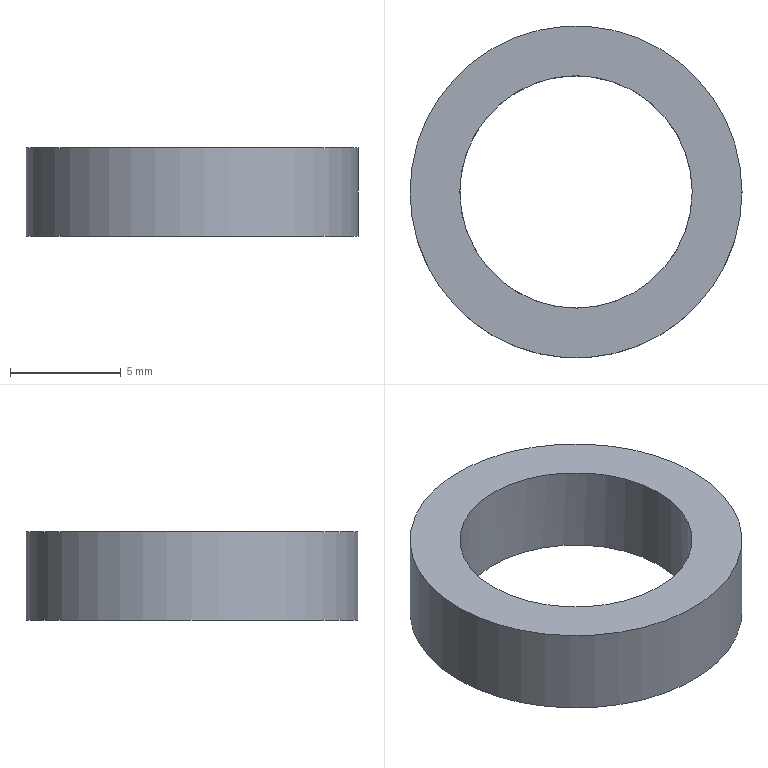Part | NX | features DATUM_CSYS 1, EXTRACT_DATUM_PLANE 1, EXTRUDE 1, SKETCH 1 | 1 solid | 4 faces | box 15 x 15 x 4 mm | volume 360.498 mm3 | cylinder 2 | plane 2 | commonest cylinder face diameters 10.5 x1 15 x1
STEP:
#1=CARTESIAN_POINT('',(-7.5,0.,4.));
#2=VERTEX_POINT('',#1);
#3=CARTESIAN_POINT('',(0.,0.,4.));
#4=DIRECTION('',(0.,0.,1.));
#5=DIRECTION('',(-1.,0.,0.));
#6=AXIS2_PLACEMENT_3D('',#3,#4,#5);
#7=CIRCLE('',#6,7.5);
#8=EDGE_CURVE('',#2,#2,#7,.T.);
#9=ORIENTED_EDGE('',*,*,#8,.F.);
#10=EDGE_LOOP('',(#9));
#11=FACE_BOUND('',#10,.T.);
#12=CARTESIAN_POINT('',(7.5,0.,0.));
#13=VERTEX_POINT('',#12);
#14=CARTESIAN_POINT('',(0.,0.,0.));
#15=DIRECTION('',(0.,0.,1.));
#16=DIRECTION('',(1.,0.,0.));
#17=AXIS2_PLACEMENT_3D('',#14,#15,#16);
#18=CIRCLE('',#17,7.5);
#19=EDGE_CURVE('',#13,#13,#18,.T.);
#20=ORIENTED_EDGE('',*,*,#19,.T.);
#21=EDGE_LOOP('',(#20));
#22=FACE_BOUND('',#21,.T.);
#23=CARTESIAN_POINT('',(0.,0.,0.));
#24=DIRECTION('',(0.,0.,1.));
#25=DIRECTION('',(1.,0.,0.));
#26=AXIS2_PLACEMENT_3D('',#23,#24,#25);
#27=CYLINDRICAL_SURFACE('',#26,7.5);
#28=ADVANCED_FACE('',(#11,#22),#27,.T.);
#29=CARTESIAN_POINT('',(-5.25,0.,4.));
#30=VERTEX_POINT('',#29);
#31=CARTESIAN_POINT('',(0.,0.,4.));
#32=DIRECTION('',(0.,0.,-1.));
#33=DIRECTION('',(-1.,0.,0.));
#34=AXIS2_PLACEMENT_3D('',#31,#32,#33);
#35=CIRCLE('',#34,5.25);
#36=EDGE_CURVE('',#30,#30,#35,.T.);
#37=ORIENTED_EDGE('',*,*,#36,.F.);
#38=EDGE_LOOP('',(#37));
#39=FACE_BOUND('',#38,.T.);
#40=CARTESIAN_POINT('',(5.25,0.,0.));
#41=VERTEX_POINT('',#40);
#42=CARTESIAN_POINT('',(0.,0.,0.));
#43=DIRECTION('',(0.,0.,-1.));
#44=DIRECTION('',(1.,0.,0.));
#45=AXIS2_PLACEMENT_3D('',#42,#43,#44);
#46=CIRCLE('',#45,5.25);
#47=EDGE_CURVE('',#41,#41,#46,.T.);
#48=ORIENTED_EDGE('',*,*,#47,.T.);
#49=EDGE_LOOP('',(#48));
#50=FACE_BOUND('',#49,.T.);
#51=CARTESIAN_POINT('',(0.,0.,0.));
#52=DIRECTION('',(0.,0.,1.));
#53=DIRECTION('',(1.,0.,0.));
#54=AXIS2_PLACEMENT_3D('',#51,#52,#53);
#55=CYLINDRICAL_SURFACE('',#54,5.25);
#56=ADVANCED_FACE('',(#39,#50),#55,.F.);
#57=ORIENTED_EDGE('',*,*,#19,.F.);
#58=EDGE_LOOP('',(#57));
#59=FACE_BOUND('',#58,.T.);
#60=ORIENTED_EDGE('',*,*,#47,.F.);
#61=EDGE_LOOP('',(#60));
#62=FACE_BOUND('',#61,.T.);
#63=CARTESIAN_POINT('',(0.,0.,0.));
#64=DIRECTION('',(0.,0.,1.));
#65=DIRECTION('',(1.,0.,0.));
#66=AXIS2_PLACEMENT_3D('',#63,#64,#65);
#67=PLANE('',#66);
#68=ADVANCED_FACE('',(#59,#62),#67,.F.);
#69=ORIENTED_EDGE('',*,*,#8,.T.);
#70=EDGE_LOOP('',(#69));
#71=FACE_BOUND('',#70,.T.);
#72=ORIENTED_EDGE('',*,*,#36,.T.);
#73=EDGE_LOOP('',(#72));
#74=FACE_BOUND('',#73,.T.);
#75=CARTESIAN_POINT('',(0.,0.,4.));
#76=DIRECTION('',(0.,0.,1.));
#77=DIRECTION('',(1.,0.,0.));
#78=AXIS2_PLACEMENT_3D('',#75,#76,#77);
#79=PLANE('',#78);
#80=ADVANCED_FACE('',(#71,#74),#79,.T.);
#81=CLOSED_SHELL('',(#28,#56,#68,#80));
#82=MANIFOLD_SOLID_BREP('',#81);
#83=(LENGTH_UNIT()NAMED_UNIT(*)SI_UNIT(.MILLI.,.METRE.));
#84=UNCERTAINTY_MEASURE_WITH_UNIT(LENGTH_MEASURE(0.00001),#83,'','');
#85=(NAMED_UNIT(*)PLANE_ANGLE_UNIT()SI_UNIT($,.RADIAN.));
#86=(NAMED_UNIT(*)SI_UNIT($,.STERADIAN.)SOLID_ANGLE_UNIT());
#87=(GEOMETRIC_REPRESENTATION_CONTEXT(3)GLOBAL_UNCERTAINTY_ASSIGNED_CONTEXT((#84))GLOBAL_UNIT_ASSIGNED_CONTEXT((#83,#85,#86))REPRESENTATION_CONTEXT('',''));
#88=ADVANCED_BREP_SHAPE_REPRESENTATION('',(#82),#87);